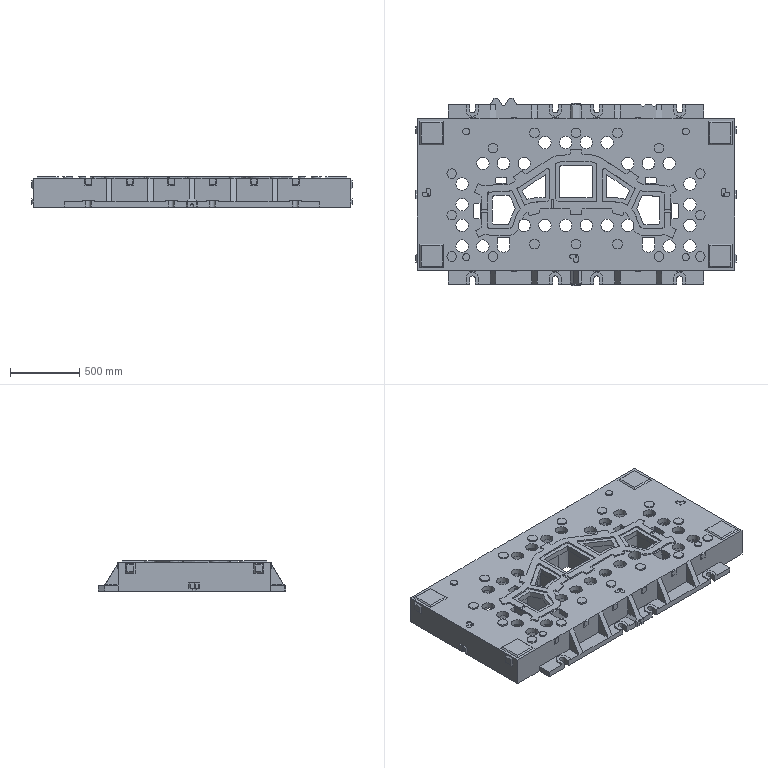Part | NX | features solid 2 | 1 solid | 741 faces | box 2320 x 1355 x 220 mm | volume 251433898 mm3 | plane 591 | cylinder 95 | spline 52 | cone 3 | commonest cylinder face diameters 90 x36 30 x19 70 x16 40 x9 10 x6 28 x4